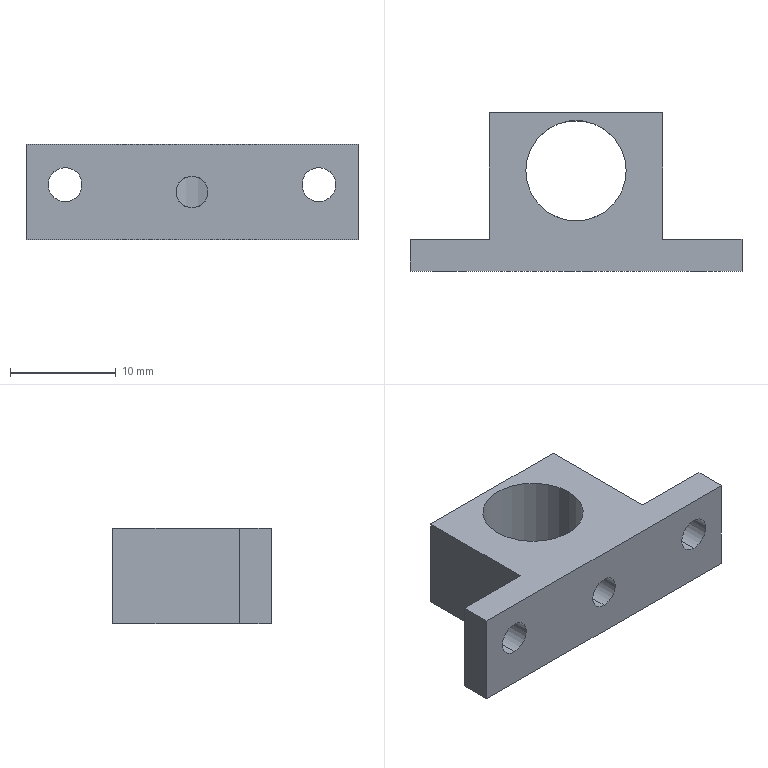Part | SolidWorks | features ICE 7, Extrusion 1 | 1 solid | 18 faces | box 31.4 x 15 x 9 mm | volume 1899 mm3 | plane 10 | cylinder 8 | commonest cylinder face diameters 3.2 x4 3 x2 9.5 x2
STEP:
#1=CARTESIAN_POINT('',(20.2,4.75,14.8));
#2=VERTEX_POINT('',#1);
#3=CARTESIAN_POINT('',(20.2,4.75,11.8));
#4=VERTEX_POINT('',#3);
#5=CARTESIAN_POINT('',(20.2,4.75,14.8));
#6=CARTESIAN_POINT('',(20.003,4.75,14.8));
#7=CARTESIAN_POINT('',(19.805,4.763,14.76));
#8=CARTESIAN_POINT('',(19.534,4.796,14.647));
#9=CARTESIAN_POINT('',(19.446,4.81,14.6));
#10=CARTESIAN_POINT('',(19.284,4.838,14.492));
#11=CARTESIAN_POINT('',(19.209,4.854,14.43));
#12=CARTESIAN_POINT('',(19.001,4.902,14.222));
#13=CARTESIAN_POINT('',(18.891,4.933,14.059));
#14=CARTESIAN_POINT('',(18.777,4.968,13.785));
#15=CARTESIAN_POINT('',(18.749,4.977,13.691));
#16=CARTESIAN_POINT('',(18.71,4.99,13.499));
#17=CARTESIAN_POINT('',(18.7,4.993,13.399));
#18=CARTESIAN_POINT('',(18.7,4.993,13.201));
#19=CARTESIAN_POINT('',(18.71,4.99,13.103));
#20=CARTESIAN_POINT('',(18.748,4.977,12.91));
#21=CARTESIAN_POINT('',(18.777,4.968,12.814));
#22=CARTESIAN_POINT('',(18.89,4.933,12.543));
#23=CARTESIAN_POINT('',(19.002,4.902,12.377));
#24=CARTESIAN_POINT('',(19.208,4.854,12.171));
#25=CARTESIAN_POINT('',(19.284,4.838,12.108));
#26=CARTESIAN_POINT('',(19.447,4.809,11.999));
#27=CARTESIAN_POINT('',(19.532,4.796,11.953));
#28=CARTESIAN_POINT('',(19.714,4.774,11.878));
#29=CARTESIAN_POINT('',(19.809,4.765,11.848));
#30=CARTESIAN_POINT('',(20.002,4.753,11.81));
#31=CARTESIAN_POINT('',(20.1,4.75,11.8));
#32=CARTESIAN_POINT('',(20.2,4.75,11.8));
#33=B_SPLINE_CURVE_WITH_KNOTS('',3,(#5,#6,#7,#8,#9,#10,#11,#12,#13,#14,#15,#16,#17,#18,#19,#20,#21,#22,#23,#24,#25,#26,#27,#28,#29,#30,#31,#32),.UNSPECIFIED.,.F.,.F.,(4,2,2,2,2,2,2,2,2,2,2,2,2,4),(0.00472,0.00531,0.005605,0.0059,0.00649,0.006785,0.00708,0.007374,0.007669,0.008259,0.008554,0.008849,0.009144,0.009439),.UNSPECIFIED.);
#34=EDGE_CURVE('',#2,#4,#33,.T.);
#35=ORIENTED_EDGE('',*,*,#34,.F.);
#36=CARTESIAN_POINT('',(20.2,0.,14.8));
#37=VERTEX_POINT('',#36);
#38=CARTESIAN_POINT('',(20.2,10.,14.8));
#39=DIRECTION('',(0.,-1.,0.));
#40=VECTOR('',#39,1000.);
#41=LINE('',#38,#40);
#42=EDGE_CURVE('',#2,#37,#41,.T.);
#43=ORIENTED_EDGE('',*,*,#42,.T.);
#44=CARTESIAN_POINT('',(20.2,0.,11.8));
#45=VERTEX_POINT('',#44);
#46=CARTESIAN_POINT('',(20.2,0.,13.3));
#47=DIRECTION('',(0.,-1.,0.));
#48=DIRECTION('',(0.,0.,-1.));
#49=AXIS2_PLACEMENT_3D('',#46,#47,#48);
#50=CIRCLE('',#49,1.5);
#51=EDGE_CURVE('',#37,#45,#50,.T.);
#52=ORIENTED_EDGE('',*,*,#51,.T.);
#53=CARTESIAN_POINT('',(20.2,10.,11.8));
#54=DIRECTION('',(0.,-1.,0.));
#55=VECTOR('',#54,1000.);
#56=LINE('',#53,#55);
#57=EDGE_CURVE('',#4,#45,#56,.T.);
#58=ORIENTED_EDGE('',*,*,#57,.F.);
#59=EDGE_LOOP('',(#35,#43,#52,#58));
#60=FACE_OUTER_BOUND('',#59,.T.);
#61=CARTESIAN_POINT('',(20.2,10.,13.3));
#62=DIRECTION('',(0.,-1.,0.));
#63=DIRECTION('',(0.,0.,-1.));
#64=AXIS2_PLACEMENT_3D('',#61,#62,#63);
#65=CYLINDRICAL_SURFACE('',#64,1.5);
#66=ADVANCED_FACE('',(#60),#65,.F.);
#67=CARTESIAN_POINT('',(20.2,4.75,11.8));
#68=CARTESIAN_POINT('',(20.3,4.75,11.8));
#69=CARTESIAN_POINT('',(20.398,4.753,11.81));
#70=CARTESIAN_POINT('',(20.59,4.765,11.848));
#71=CARTESIAN_POINT('',(20.686,4.774,11.878));
#72=CARTESIAN_POINT('',(20.867,4.796,11.953));
#73=CARTESIAN_POINT('',(20.953,4.809,11.999));
#74=CARTESIAN_POINT('',(21.116,4.838,12.108));
#75=CARTESIAN_POINT('',(21.192,4.854,12.171));
#76=CARTESIAN_POINT('',(21.398,4.902,12.377));
#77=CARTESIAN_POINT('',(21.51,4.934,12.543));
#78=CARTESIAN_POINT('',(21.66,4.979,12.904));
#79=CARTESIAN_POINT('',(21.7,4.993,13.102));
#80=CARTESIAN_POINT('',(21.7,4.993,13.398));
#81=CARTESIAN_POINT('',(21.69,4.99,13.498));
#82=CARTESIAN_POINT('',(21.652,4.977,13.691));
#83=CARTESIAN_POINT('',(21.623,4.968,13.785));
#84=CARTESIAN_POINT('',(21.509,4.933,14.058));
#85=CARTESIAN_POINT('',(21.399,4.902,14.223));
#86=CARTESIAN_POINT('',(21.191,4.854,14.43));
#87=CARTESIAN_POINT('',(21.116,4.838,14.492));
#88=CARTESIAN_POINT('',(20.954,4.809,14.6));
#89=CARTESIAN_POINT('',(20.866,4.796,14.648));
#90=CARTESIAN_POINT('',(20.595,4.763,14.76));
#91=CARTESIAN_POINT('',(20.397,4.75,14.8));
#92=CARTESIAN_POINT('',(20.2,4.75,14.8));
#93=B_SPLINE_CURVE_WITH_KNOTS('',3,(#67,#68,#69,#70,#71,#72,#73,#74,#75,#76,#77,#78,#79,#80,#81,#82,#83,#84,#85,#86,#87,#88,#89,#90,#91,#92),.UNSPECIFIED.,.F.,.F.,(4,2,2,2,2,2,2,2,2,2,2,2,4),(0.,0.000295,0.00059,0.000885,0.00118,0.00177,0.00236,0.002655,0.00295,0.00354,0.003835,0.00413,0.00472),.UNSPECIFIED.);
#94=EDGE_CURVE('',#4,#2,#93,.T.);
#95=ORIENTED_EDGE('',*,*,#94,.T.);
#96=ORIENTED_EDGE('',*,*,#34,.T.);
#97=EDGE_LOOP('',(#95,#96));
#98=FACE_BOUND('',#97,.T.);
#99=CARTESIAN_POINT('',(24.95,9.5,8.8));
#100=VERTEX_POINT('',#99);
#101=CARTESIAN_POINT('',(15.45,9.5,8.8));
#102=VERTEX_POINT('',#101);
#103=CARTESIAN_POINT('',(20.2,9.5,8.8));
#104=DIRECTION('',(0.,0.,-1.));
#105=DIRECTION('',(1.,0.,0.));
#106=AXIS2_PLACEMENT_3D('',#103,#104,#105);
#107=CIRCLE('',#106,4.75);
#108=EDGE_CURVE('',#100,#102,#107,.T.);
#109=ORIENTED_EDGE('',*,*,#108,.T.);
#110=CARTESIAN_POINT('',(15.45,9.5,17.8));
#111=VERTEX_POINT('',#110);
#112=CARTESIAN_POINT('',(15.45,9.5,-16.));
#113=DIRECTION('',(0.,0.,1.));
#114=VECTOR('',#113,1000.);
#115=LINE('',#112,#114);
#116=EDGE_CURVE('',#102,#111,#115,.T.);
#117=ORIENTED_EDGE('',*,*,#116,.T.);
#118=CARTESIAN_POINT('',(24.95,9.5,17.8));
#119=VERTEX_POINT('',#118);
#120=CARTESIAN_POINT('',(20.2,9.5,17.8));
#121=DIRECTION('',(0.,0.,1.));
#122=DIRECTION('',(-1.,0.,0.));
#123=AXIS2_PLACEMENT_3D('',#120,#121,#122);
#124=CIRCLE('',#123,4.75);
#125=EDGE_CURVE('',#111,#119,#124,.T.);
#126=ORIENTED_EDGE('',*,*,#125,.T.);
#127=CARTESIAN_POINT('',(24.95,9.5,-16.));
#128=DIRECTION('',(0.,0.,1.));
#129=VECTOR('',#128,1000.);
#130=LINE('',#127,#129);
#131=EDGE_CURVE('',#100,#119,#130,.T.);
#132=ORIENTED_EDGE('',*,*,#131,.F.);
#133=EDGE_LOOP('',(#109,#117,#126,#132));
#134=FACE_OUTER_BOUND('',#133,.T.);
#135=CARTESIAN_POINT('',(20.2,9.5,-16.));
#136=DIRECTION('',(0.,0.,1.));
#137=DIRECTION('',(1.,0.,0.));
#138=AXIS2_PLACEMENT_3D('',#135,#136,#137);
#139=CYLINDRICAL_SURFACE('',#138,4.75);
#140=ADVANCED_FACE('',(#98,#134),#139,.F.);
#141=CARTESIAN_POINT('',(8.2,0.,12.4));
#142=VERTEX_POINT('',#141);
#143=CARTESIAN_POINT('',(8.2,0.,15.6));
#144=VERTEX_POINT('',#143);
#145=CARTESIAN_POINT('',(8.2,0.,14.));
#146=DIRECTION('',(0.,1.,0.));
#147=DIRECTION('',(0.,0.,1.));
#148=AXIS2_PLACEMENT_3D('',#145,#146,#147);
#149=CIRCLE('',#148,1.6);
#150=EDGE_CURVE('',#142,#144,#149,.T.);
#151=ORIENTED_EDGE('',*,*,#150,.F.);
#152=CARTESIAN_POINT('',(8.2,3.,12.4));
#153=VERTEX_POINT('',#152);
#154=CARTESIAN_POINT('',(8.2,-21.,12.4));
#155=DIRECTION('',(0.,1.,0.));
#156=VECTOR('',#155,1000.);
#157=LINE('',#154,#156);
#158=EDGE_CURVE('',#142,#153,#157,.T.);
#159=ORIENTED_EDGE('',*,*,#158,.T.);
#160=CARTESIAN_POINT('',(8.2,3.,15.6));
#161=VERTEX_POINT('',#160);
#162=CARTESIAN_POINT('',(8.2,3.,14.));
#163=DIRECTION('',(0.,-1.,0.));
#164=DIRECTION('',(0.,0.,1.));
#165=AXIS2_PLACEMENT_3D('',#162,#163,#164);
#166=CIRCLE('',#165,1.6);
#167=EDGE_CURVE('',#161,#153,#166,.T.);
#168=ORIENTED_EDGE('',*,*,#167,.F.);
#169=CARTESIAN_POINT('',(8.2,-21.,15.6));
#170=DIRECTION('',(0.,1.,0.));
#171=VECTOR('',#170,1000.);
#172=LINE('',#169,#171);
#173=EDGE_CURVE('',#144,#161,#172,.T.);
#174=ORIENTED_EDGE('',*,*,#173,.F.);
#175=EDGE_LOOP('',(#151,#159,#168,#174));
#176=FACE_OUTER_BOUND('',#175,.T.);
#177=CARTESIAN_POINT('',(8.2,-21.,14.));
#178=DIRECTION('',(0.,1.,0.));
#179=DIRECTION('',(0.,0.,1.));
#180=AXIS2_PLACEMENT_3D('',#177,#178,#179);
#181=CYLINDRICAL_SURFACE('',#180,1.6);
#182=ADVANCED_FACE('',(#176),#181,.F.);
#183=CARTESIAN_POINT('',(32.2,0.,12.4));
#184=VERTEX_POINT('',#183);
#185=CARTESIAN_POINT('',(32.2,0.,15.6));
#186=VERTEX_POINT('',#185);
#187=CARTESIAN_POINT('',(32.2,0.,14.));
#188=DIRECTION('',(0.,1.,0.));
#189=DIRECTION('',(0.,0.,1.));
#190=AXIS2_PLACEMENT_3D('',#187,#188,#189);
#191=CIRCLE('',#190,1.6);
#192=EDGE_CURVE('',#184,#186,#191,.T.);
#193=ORIENTED_EDGE('',*,*,#192,.F.);
#194=CARTESIAN_POINT('',(32.2,3.,12.4));
#195=VERTEX_POINT('',#194);
#196=CARTESIAN_POINT('',(32.2,-21.,12.4));
#197=DIRECTION('',(0.,1.,0.));
#198=VECTOR('',#197,1000.);
#199=LINE('',#196,#198);
#200=EDGE_CURVE('',#184,#195,#199,.T.);
#201=ORIENTED_EDGE('',*,*,#200,.T.);
#202=CARTESIAN_POINT('',(32.2,3.,15.6));
#203=VERTEX_POINT('',#202);
#204=CARTESIAN_POINT('',(32.2,3.,14.));
#205=DIRECTION('',(0.,-1.,0.));
#206=DIRECTION('',(0.,0.,1.));
#207=AXIS2_PLACEMENT_3D('',#204,#205,#206);
#208=CIRCLE('',#207,1.6);
#209=EDGE_CURVE('',#203,#195,#208,.T.);
#210=ORIENTED_EDGE('',*,*,#209,.F.);
#211=CARTESIAN_POINT('',(32.2,-21.,15.6));
#212=DIRECTION('',(0.,1.,0.));
#213=VECTOR('',#212,1000.);
#214=LINE('',#211,#213);
#215=EDGE_CURVE('',#186,#203,#214,.T.);
#216=ORIENTED_EDGE('',*,*,#215,.F.);
#217=EDGE_LOOP('',(#193,#201,#210,#216));
#218=FACE_OUTER_BOUND('',#217,.T.);
#219=CARTESIAN_POINT('',(32.2,-21.,14.));
#220=DIRECTION('',(0.,1.,0.));
#221=DIRECTION('',(0.,0.,1.));
#222=AXIS2_PLACEMENT_3D('',#219,#220,#221);
#223=CYLINDRICAL_SURFACE('',#222,1.6);
#224=ADVANCED_FACE('',(#218),#223,.F.);
#225=ORIENTED_EDGE('',*,*,#200,.F.);
#226=CARTESIAN_POINT('',(32.2,0.,14.));
#227=DIRECTION('',(0.,1.,0.));
#228=DIRECTION('',(0.,0.,1.));
#229=AXIS2_PLACEMENT_3D('',#226,#227,#228);
#230=CIRCLE('',#229,1.6);
#231=EDGE_CURVE('',#186,#184,#230,.T.);
#232=ORIENTED_EDGE('',*,*,#231,.F.);
#233=ORIENTED_EDGE('',*,*,#215,.T.);
#234=CARTESIAN_POINT('',(32.2,3.,14.));
#235=DIRECTION('',(0.,-1.,0.));
#236=DIRECTION('',(0.,0.,1.));
#237=AXIS2_PLACEMENT_3D('',#234,#235,#236);
#238=CIRCLE('',#237,1.6);
#239=EDGE_CURVE('',#195,#203,#238,.T.);
#240=ORIENTED_EDGE('',*,*,#239,.F.);
#241=EDGE_LOOP('',(#225,#232,#233,#240));
#242=FACE_OUTER_BOUND('',#241,.T.);
#243=CARTESIAN_POINT('',(32.2,-21.,14.));
#244=DIRECTION('',(0.,1.,0.));
#245=DIRECTION('',(0.,0.,1.));
#246=AXIS2_PLACEMENT_3D('',#243,#244,#245);
#247=CYLINDRICAL_SURFACE('',#246,1.6);
#248=ADVANCED_FACE('',(#242),#247,.F.);
#249=ORIENTED_EDGE('',*,*,#158,.F.);
#250=CARTESIAN_POINT('',(8.2,0.,14.));
#251=DIRECTION('',(0.,1.,0.));
#252=DIRECTION('',(0.,0.,1.));
#253=AXIS2_PLACEMENT_3D('',#250,#251,#252);
#254=CIRCLE('',#253,1.6);
#255=EDGE_CURVE('',#144,#142,#254,.T.);
#256=ORIENTED_EDGE('',*,*,#255,.F.);
#257=ORIENTED_EDGE('',*,*,#173,.T.);
#258=CARTESIAN_POINT('',(8.2,3.,14.));
#259=DIRECTION('',(0.,-1.,0.));
#260=DIRECTION('',(0.,0.,1.));
#261=AXIS2_PLACEMENT_3D('',#258,#259,#260);
#262=CIRCLE('',#261,1.6);
#263=EDGE_CURVE('',#153,#161,#262,.T.);
#264=ORIENTED_EDGE('',*,*,#263,.F.);
#265=EDGE_LOOP('',(#249,#256,#257,#264));
#266=FACE_OUTER_BOUND('',#265,.T.);
#267=CARTESIAN_POINT('',(8.2,-21.,14.));
#268=DIRECTION('',(0.,1.,0.));
#269=DIRECTION('',(0.,0.,1.));
#270=AXIS2_PLACEMENT_3D('',#267,#268,#269);
#271=CYLINDRICAL_SURFACE('',#270,1.6);
#272=ADVANCED_FACE('',(#266),#271,.F.);
#273=CARTESIAN_POINT('',(12.,15.,17.8));
#274=VERTEX_POINT('',#273);
#275=CARTESIAN_POINT('',(12.,15.,8.8));
#276=VERTEX_POINT('',#275);
#277=CARTESIAN_POINT('',(12.,15.,8.8));
#278=DIRECTION('',(0.,0.,-1.));
#279=VECTOR('',#278,1000.);
#280=LINE('',#277,#279);
#281=EDGE_CURVE('',#274,#276,#280,.T.);
#282=ORIENTED_EDGE('',*,*,#281,.F.);
#283=CARTESIAN_POINT('',(28.4,15.,17.8));
#284=VERTEX_POINT('',#283);
#285=CARTESIAN_POINT('',(0.,15.,17.8));
#286=DIRECTION('',(-1.,0.,0.));
#287=VECTOR('',#286,1000.);
#288=LINE('',#285,#287);
#289=EDGE_CURVE('',#284,#274,#288,.T.);
#290=ORIENTED_EDGE('',*,*,#289,.F.);
#291=CARTESIAN_POINT('',(28.4,15.,8.8));
#292=VERTEX_POINT('',#291);
#293=CARTESIAN_POINT('',(28.4,15.,17.8));
#294=DIRECTION('',(0.,0.,1.));
#295=VECTOR('',#294,1000.);
#296=LINE('',#293,#295);
#297=EDGE_CURVE('',#292,#284,#296,.T.);
#298=ORIENTED_EDGE('',*,*,#297,.F.);
#299=CARTESIAN_POINT('',(40.4,15.,8.8));
#300=DIRECTION('',(1.,0.,0.));
#301=VECTOR('',#300,1000.);
#302=LINE('',#299,#301);
#303=EDGE_CURVE('',#276,#292,#302,.T.);
#304=ORIENTED_EDGE('',*,*,#303,.F.);
#305=EDGE_LOOP('',(#282,#290,#298,#304));
#306=FACE_OUTER_BOUND('',#305,.T.);
#307=CARTESIAN_POINT('',(0.,15.,0.));
#308=DIRECTION('',(0.,1.,0.));
#309=DIRECTION('',(0.,0.,1.));
#310=AXIS2_PLACEMENT_3D('',#307,#308,#309);
#311=PLANE('',#310);
#312=ADVANCED_FACE('',(#306),#311,.T.);
#313=CARTESIAN_POINT('',(20.2,0.,13.3));
#314=DIRECTION('',(0.,-1.,0.));
#315=DIRECTION('',(0.,0.,-1.));
#316=AXIS2_PLACEMENT_3D('',#313,#314,#315);
#317=CIRCLE('',#316,1.5);
#318=EDGE_CURVE('',#45,#37,#317,.T.);
#319=ORIENTED_EDGE('',*,*,#318,.F.);
#320=ORIENTED_EDGE('',*,*,#51,.F.);
#321=EDGE_LOOP('',(#319,#320));
#322=FACE_BOUND('',#321,.T.);
#323=ORIENTED_EDGE('',*,*,#255,.T.);
#324=ORIENTED_EDGE('',*,*,#150,.T.);
#325=EDGE_LOOP('',(#323,#324));
#326=FACE_BOUND('',#325,.T.);
#327=ORIENTED_EDGE('',*,*,#231,.T.);
#328=ORIENTED_EDGE('',*,*,#192,.T.);
#329=EDGE_LOOP('',(#327,#328));
#330=FACE_BOUND('',#329,.T.);
#331=CARTESIAN_POINT('',(35.9,0.,17.8));
#332=VERTEX_POINT('',#331);
#333=CARTESIAN_POINT('',(4.5,0.,17.8));
#334=VERTEX_POINT('',#333);
#335=CARTESIAN_POINT('',(0.,0.,17.8));
#336=DIRECTION('',(-1.,0.,0.));
#337=VECTOR('',#336,1000.);
#338=LINE('',#335,#337);
#339=EDGE_CURVE('',#332,#334,#338,.T.);
#340=ORIENTED_EDGE('',*,*,#339,.T.);
#341=CARTESIAN_POINT('',(4.5,0.,8.8));
#342=VERTEX_POINT('',#341);
#343=CARTESIAN_POINT('',(4.5,0.,0.));
#344=DIRECTION('',(0.,0.,-1.));
#345=VECTOR('',#344,1000.);
#346=LINE('',#343,#345);
#347=EDGE_CURVE('',#334,#342,#346,.T.);
#348=ORIENTED_EDGE('',*,*,#347,.T.);
#349=CARTESIAN_POINT('',(35.9,0.,8.8));
#350=VERTEX_POINT('',#349);
#351=CARTESIAN_POINT('',(0.,0.,8.8));
#352=DIRECTION('',(1.,0.,0.));
#353=VECTOR('',#352,1000.);
#354=LINE('',#351,#353);
#355=EDGE_CURVE('',#342,#350,#354,.T.);
#356=ORIENTED_EDGE('',*,*,#355,.T.);
#357=CARTESIAN_POINT('',(35.9,0.,0.));
#358=DIRECTION('',(0.,0.,1.));
#359=VECTOR('',#358,1000.);
#360=LINE('',#357,#359);
#361=EDGE_CURVE('',#350,#332,#360,.T.);
#362=ORIENTED_EDGE('',*,*,#361,.T.);
#363=EDGE_LOOP('',(#340,#348,#356,#362));
#364=FACE_OUTER_BOUND('',#363,.T.);
#365=CARTESIAN_POINT('',(0.,0.,0.));
#366=DIRECTION('',(0.,1.,0.));
#367=DIRECTION('',(0.,0.,1.));
#368=AXIS2_PLACEMENT_3D('',#365,#366,#367);
#369=PLANE('',#368);
#370=ADVANCED_FACE('',(#322,#326,#330,#364),#369,.F.);
#371=ORIENTED_EDGE('',*,*,#116,.F.);
#372=CARTESIAN_POINT('',(20.2,9.5,8.8));
#373=DIRECTION('',(0.,0.,-1.));
#374=DIRECTION('',(1.,0.,0.));
#375=AXIS2_PLACEMENT_3D('',#372,#373,#374);
#376=CIRCLE('',#375,4.75);
#377=EDGE_CURVE('',#102,#100,#376,.T.);
#378=ORIENTED_EDGE('',*,*,#377,.T.);
#379=ORIENTED_EDGE('',*,*,#131,.T.);
#380=CARTESIAN_POINT('',(20.2,9.5,17.8));
#381=DIRECTION('',(0.,0.,1.));
#382=DIRECTION('',(-1.,0.,0.));
#383=AXIS2_PLACEMENT_3D('',#380,#381,#382);
#384=CIRCLE('',#383,4.75);
#385=EDGE_CURVE('',#119,#111,#384,.T.);
#386=ORIENTED_EDGE('',*,*,#385,.T.);
#387=EDGE_LOOP('',(#371,#378,#379,#386));
#388=FACE_OUTER_BOUND('',#387,.T.);
#389=CARTESIAN_POINT('',(20.2,9.5,-16.));
#390=DIRECTION('',(0.,0.,1.));
#391=DIRECTION('',(1.,0.,0.));
#392=AXIS2_PLACEMENT_3D('',#389,#390,#391);
#393=CYLINDRICAL_SURFACE('',#392,4.75);
#394=ADVANCED_FACE('',(#388),#393,.F.);
#395=ORIENTED_EDGE('',*,*,#108,.F.);
#396=ORIENTED_EDGE('',*,*,#377,.F.);
#397=EDGE_LOOP('',(#395,#396));
#398=FACE_BOUND('',#397,.T.);
#399=ORIENTED_EDGE('',*,*,#355,.F.);
#400=CARTESIAN_POINT('',(4.5,3.,8.8));
#401=VERTEX_POINT('',#400);
#402=CARTESIAN_POINT('',(4.5,-9.,8.8));
#403=DIRECTION('',(0.,1.,0.));
#404=VECTOR('',#403,1000.);
#405=LINE('',#402,#404);
#406=EDGE_CURVE('',#342,#401,#405,.T.);
#407=ORIENTED_EDGE('',*,*,#406,.T.);
#408=CARTESIAN_POINT('',(12.,3.,8.8));
#409=VERTEX_POINT('',#408);
#410=CARTESIAN_POINT('',(0.,3.,8.8));
#411=DIRECTION('',(-1.,0.,0.));
#412=VECTOR('',#411,1000.);
#413=LINE('',#410,#412);
#414=EDGE_CURVE('',#409,#401,#413,.T.);
#415=ORIENTED_EDGE('',*,*,#414,.F.);
#416=CARTESIAN_POINT('',(12.,3.,8.8));
#417=DIRECTION('',(0.,1.,0.));
#418=VECTOR('',#417,1000.);
#419=LINE('',#416,#418);
#420=EDGE_CURVE('',#409,#276,#419,.T.);
#421=ORIENTED_EDGE('',*,*,#420,.T.);
#422=ORIENTED_EDGE('',*,*,#303,.T.);
#423=CARTESIAN_POINT('',(28.4,3.,8.8));
#424=VERTEX_POINT('',#423);
#425=CARTESIAN_POINT('',(28.4,3.,8.8));
#426=DIRECTION('',(0.,1.,0.));
#427=VECTOR('',#426,1000.);
#428=LINE('',#425,#427);
#429=EDGE_CURVE('',#424,#292,#428,.T.);
#430=ORIENTED_EDGE('',*,*,#429,.F.);
#431=CARTESIAN_POINT('',(35.9,3.,8.8));
#432=VERTEX_POINT('',#431);
#433=CARTESIAN_POINT('',(40.4,3.,8.8));
#434=DIRECTION('',(-1.,0.,0.));
#435=VECTOR('',#434,1000.);
#436=LINE('',#433,#435);
#437=EDGE_CURVE('',#432,#424,#436,.T.);
#438=ORIENTED_EDGE('',*,*,#437,.F.);
#439=CARTESIAN_POINT('',(35.9,-9.,8.8));
#440=DIRECTION('',(0.,1.,0.));
#441=VECTOR('',#440,1000.);
#442=LINE('',#439,#441);
#443=EDGE_CURVE('',#350,#432,#442,.T.);
#444=ORIENTED_EDGE('',*,*,#443,.F.);
#445=EDGE_LOOP('',(#399,#407,#415,#421,#422,#430,#438,#444));
#446=FACE_OUTER_BOUND('',#445,.T.);
#447=CARTESIAN_POINT('',(40.4,-21.,8.8));
#448=DIRECTION('',(0.,0.,1.));
#449=DIRECTION('',(1.,0.,0.));
#450=AXIS2_PLACEMENT_3D('',#447,#448,#449);
#451=PLANE('',#450);
#452=ADVANCED_FACE('',(#398,#446),#451,.F.);
#453=ORIENTED_EDGE('',*,*,#385,.F.);
#454=ORIENTED_EDGE('',*,*,#125,.F.);
#455=EDGE_LOOP('',(#453,#454));
#456=FACE_BOUND('',#455,.T.);
#457=CARTESIAN_POINT('',(4.5,3.,17.8));
#458=VERTEX_POINT('',#457);
#459=CARTESIAN_POINT('',(12.,3.,17.8));
#460=VERTEX_POINT('',#459);
#461=CARTESIAN_POINT('',(0.,3.,17.8));
#462=DIRECTION('',(1.,0.,0.));
#463=VECTOR('',#462,1000.);
#464=LINE('',#461,#463);
#465=EDGE_CURVE('',#458,#460,#464,.T.);
#466=ORIENTED_EDGE('',*,*,#465,.F.);
#467=CARTESIAN_POINT('',(4.5,-9.,17.8));
#468=DIRECTION('',(0.,1.,0.));
#469=VECTOR('',#468,1000.);
#470=LINE('',#467,#469);
#471=EDGE_CURVE('',#334,#458,#470,.T.);
#472=ORIENTED_EDGE('',*,*,#471,.F.);
#473=ORIENTED_EDGE('',*,*,#339,.F.);
#474=CARTESIAN_POINT('',(35.9,3.,17.8));
#475=VERTEX_POINT('',#474);
#476=CARTESIAN_POINT('',(35.9,-9.,17.8));
#477=DIRECTION('',(0.,1.,0.));
#478=VECTOR('',#477,1000.);
#479=LINE('',#476,#478);
#480=EDGE_CURVE('',#332,#475,#479,.T.);
#481=ORIENTED_EDGE('',*,*,#480,.T.);
#482=CARTESIAN_POINT('',(28.4,3.,17.8));
#483=VERTEX_POINT('',#482);
#484=CARTESIAN_POINT('',(40.4,3.,17.8));
#485=DIRECTION('',(1.,0.,0.));
#486=VECTOR('',#485,1000.);
#487=LINE('',#484,#486);
#488=EDGE_CURVE('',#483,#475,#487,.T.);
#489=ORIENTED_EDGE('',*,*,#488,.F.);
#490=CARTESIAN_POINT('',(28.4,3.,17.8));
#491=DIRECTION('',(0.,1.,0.));
#492=VECTOR('',#491,1000.);
#493=LINE('',#490,#492);
#494=EDGE_CURVE('',#483,#284,#493,.T.);
#495=ORIENTED_EDGE('',*,*,#494,.T.);
#496=ORIENTED_EDGE('',*,*,#289,.T.);
#497=CARTESIAN_POINT('',(12.,3.,17.8));
#498=DIRECTION('',(0.,1.,0.));
#499=VECTOR('',#498,1000.);
#500=LINE('',#497,#499);
#501=EDGE_CURVE('',#460,#274,#500,.T.);
#502=ORIENTED_EDGE('',*,*,#501,.F.);
#503=EDGE_LOOP('',(#466,#472,#473,#481,#489,#495,#496,#502));
#504=FACE_OUTER_BOUND('',#503,.T.);
#505=CARTESIAN_POINT('',(0.,-21.,17.8));
#506=DIRECTION('',(0.,0.,-1.));
#507=DIRECTION('',(-1.,0.,0.));
#508=AXIS2_PLACEMENT_3D('',#505,#506,#507);
#509=PLANE('',#508);
#510=ADVANCED_FACE('',(#456,#504),#509,.F.);
#511=CARTESIAN_POINT('',(35.9,3.,17.8));
#512=DIRECTION('',(0.,0.,1.));
#513=VECTOR('',#512,1000.);
#514=LINE('',#511,#513);
#515=EDGE_CURVE('',#432,#475,#514,.T.);
#516=ORIENTED_EDGE('',*,*,#515,.F.);
#517=ORIENTED_EDGE('',*,*,#437,.T.);
#518=CARTESIAN_POINT('',(28.4,3.,17.8));
#519=DIRECTION('',(0.,0.,1.));
#520=VECTOR('',#519,1000.);
#521=LINE('',#518,#520);
#522=EDGE_CURVE('',#424,#483,#521,.T.);
#523=ORIENTED_EDGE('',*,*,#522,.T.);
#524=ORIENTED_EDGE('',*,*,#488,.T.);
#525=EDGE_LOOP('',(#516,#517,#523,#524));
#526=FACE_OUTER_BOUND('',#525,.T.);
#527=ORIENTED_EDGE('',*,*,#209,.T.);
#528=ORIENTED_EDGE('',*,*,#239,.T.);
#529=EDGE_LOOP('',(#527,#528));
#530=FACE_BOUND('',#529,.T.);
#531=CARTESIAN_POINT('',(0.,3.,0.));
#532=DIRECTION('',(0.,1.,0.));
#533=DIRECTION('',(0.,0.,1.));
#534=AXIS2_PLACEMENT_3D('',#531,#532,#533);
#535=PLANE('',#534);
#536=ADVANCED_FACE('',(#526,#530),#535,.T.);
#537=ORIENTED_EDGE('',*,*,#297,.T.);
#538=ORIENTED_EDGE('',*,*,#494,.F.);
#539=ORIENTED_EDGE('',*,*,#522,.F.);
#540=ORIENTED_EDGE('',*,*,#429,.T.);
#541=EDGE_LOOP('',(#537,#538,#539,#540));
#542=FACE_OUTER_BOUND('',#541,.T.);
#543=CARTESIAN_POINT('',(28.4,3.,17.8));
#544=DIRECTION('',(-1.,0.,0.));
#545=DIRECTION('',(0.,0.,1.));
#546=AXIS2_PLACEMENT_3D('',#543,#544,#545);
#547=PLANE('',#546);
#548=ADVANCED_FACE('',(#542),#547,.F.);
#549=CARTESIAN_POINT('',(4.5,3.,8.8));
#550=DIRECTION('',(0.,0.,-1.));
#551=VECTOR('',#550,1000.);
#552=LINE('',#549,#551);
#553=EDGE_CURVE('',#458,#401,#552,.T.);
#554=ORIENTED_EDGE('',*,*,#553,.F.);
#555=ORIENTED_EDGE('',*,*,#465,.T.);
#556=CARTESIAN_POINT('',(12.,3.,8.8));
#557=DIRECTION('',(0.,0.,-1.));
#558=VECTOR('',#557,1000.);
#559=LINE('',#556,#558);
#560=EDGE_CURVE('',#460,#409,#559,.T.);
#561=ORIENTED_EDGE('',*,*,#560,.T.);
#562=ORIENTED_EDGE('',*,*,#414,.T.);
#563=EDGE_LOOP('',(#554,#555,#561,#562));
#564=FACE_OUTER_BOUND('',#563,.T.);
#565=ORIENTED_EDGE('',*,*,#167,.T.);
#566=ORIENTED_EDGE('',*,*,#263,.T.);
#567=EDGE_LOOP('',(#565,#566));
#568=FACE_BOUND('',#567,.T.);
#569=CARTESIAN_POINT('',(0.,3.,0.));
#570=DIRECTION('',(0.,1.,0.));
#571=DIRECTION('',(0.,0.,1.));
#572=AXIS2_PLACEMENT_3D('',#569,#570,#571);
#573=PLANE('',#572);
#574=ADVANCED_FACE('',(#564,#568),#573,.T.);
#575=ORIENTED_EDGE('',*,*,#281,.T.);
#576=ORIENTED_EDGE('',*,*,#420,.F.);
#577=ORIENTED_EDGE('',*,*,#560,.F.);
#578=ORIENTED_EDGE('',*,*,#501,.T.);
#579=EDGE_LOOP('',(#575,#576,#577,#578));
#580=FACE_OUTER_BOUND('',#579,.T.);
#581=CARTESIAN_POINT('',(12.,3.,8.8));
#582=DIRECTION('',(1.,0.,0.));
#583=DIRECTION('',(0.,0.,-1.));
#584=AXIS2_PLACEMENT_3D('',#581,#582,#583);
#585=PLANE('',#584);
#586=ADVANCED_FACE('',(#580),#585,.F.);
#587=ORIENTED_EDGE('',*,*,#471,.T.);
#588=ORIENTED_EDGE('',*,*,#553,.T.);
#589=ORIENTED_EDGE('',*,*,#406,.F.);
#590=ORIENTED_EDGE('',*,*,#347,.F.);
#591=EDGE_LOOP('',(#587,#588,#589,#590));
#592=FACE_OUTER_BOUND('',#591,.T.);
#593=CARTESIAN_POINT('',(4.5,-9.,8.8));
#594=DIRECTION('',(1.,0.,0.));
#595=DIRECTION('',(0.,0.,-1.));
#596=AXIS2_PLACEMENT_3D('',#593,#594,#595);
#597=PLANE('',#596);
#598=ADVANCED_FACE('',(#592),#597,.F.);
#599=ORIENTED_EDGE('',*,*,#443,.T.);
#600=ORIENTED_EDGE('',*,*,#515,.T.);
#601=ORIENTED_EDGE('',*,*,#480,.F.);
#602=ORIENTED_EDGE('',*,*,#361,.F.);
#603=EDGE_LOOP('',(#599,#600,#601,#602));
#604=FACE_OUTER_BOUND('',#603,.T.);
#605=CARTESIAN_POINT('',(35.9,-9.,17.8));
#606=DIRECTION('',(-1.,0.,0.));
#607=DIRECTION('',(0.,0.,1.));
#608=AXIS2_PLACEMENT_3D('',#605,#606,#607);
#609=PLANE('',#608);
#610=ADVANCED_FACE('',(#604),#609,.F.);
#611=ORIENTED_EDGE('',*,*,#42,.F.);
#612=ORIENTED_EDGE('',*,*,#94,.F.);
#613=ORIENTED_EDGE('',*,*,#57,.T.);
#614=ORIENTED_EDGE('',*,*,#318,.T.);
#615=EDGE_LOOP('',(#611,#612,#613,#614));
#616=FACE_OUTER_BOUND('',#615,.T.);
#617=CARTESIAN_POINT('',(20.2,10.,13.3));
#618=DIRECTION('',(0.,-1.,0.));
#619=DIRECTION('',(0.,0.,-1.));
#620=AXIS2_PLACEMENT_3D('',#617,#618,#619);
#621=CYLINDRICAL_SURFACE('',#620,1.5);
#622=ADVANCED_FACE('',(#616),#621,.F.);
#623=CLOSED_SHELL('',(#66,#140,#182,#224,#248,#272,#312,#370,#394,#452,#510,#536,#548,#574,#586,#598,#610,#622));
#624=MANIFOLD_SOLID_BREP('',#623);
#625=CARTESIAN_POINT('',(0.,0.,0.));
#626=DIRECTION('',(0.,0.,1.));
#627=DIRECTION('',(1.,0.,0.));
#628=AXIS2_PLACEMENT_3D('',#625,#626,#627);
#629=(LENGTH_UNIT()NAMED_UNIT(*)SI_UNIT(.MILLI.,.METRE.));
#630=UNCERTAINTY_MEASURE_WITH_UNIT(LENGTH_MEASURE(0.00001),#629,'','');
#631=(NAMED_UNIT(*)PLANE_ANGLE_UNIT()SI_UNIT($,.RADIAN.));
#632=(NAMED_UNIT(*)SI_UNIT($,.STERADIAN.)SOLID_ANGLE_UNIT());
#633=(GEOMETRIC_REPRESENTATION_CONTEXT(3)GLOBAL_UNCERTAINTY_ASSIGNED_CONTEXT((#630))GLOBAL_UNIT_ASSIGNED_CONTEXT((#629,#631,#632))REPRESENTATION_CONTEXT('',''));
#634=ADVANCED_BREP_SHAPE_REPRESENTATION('',(#624,#628),#633);